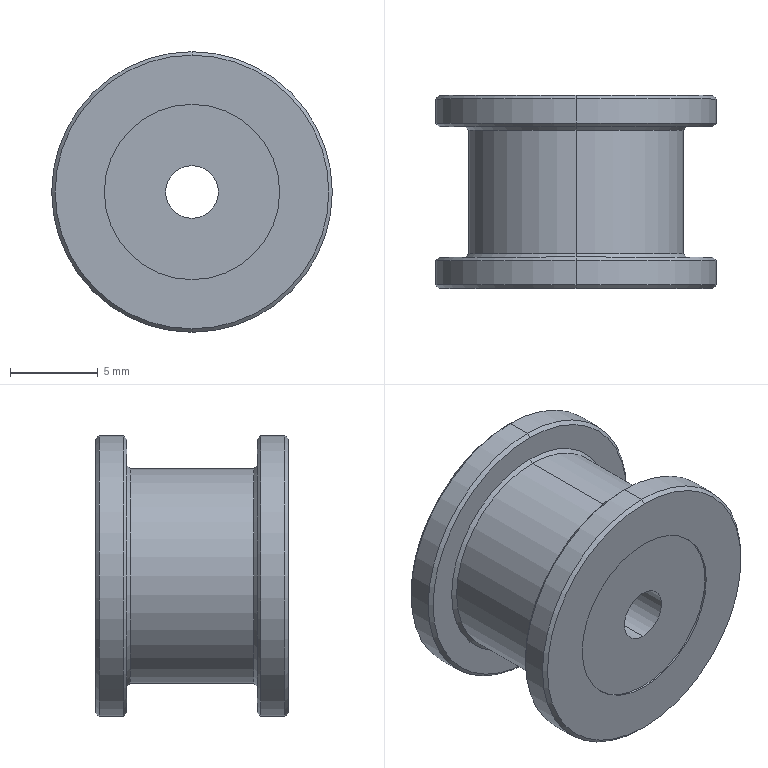Part | SolidWorks | features BaseBody 1 | 1 solid | 30 faces | box 16 x 11 x 16 mm | volume 1494 mm3 | cylinder 12 | cone 12 | plane 6 | commonest cylinder face diameters 10 x4 16 x4 3 x2 12.22 x2
STEP:
#1=CARTESIAN_POINT('',(-150.906,17.76,6.11));
#2=VERTEX_POINT('',#1);
#3=CARTESIAN_POINT('',(-150.906,17.76,-6.11));
#4=VERTEX_POINT('',#3);
#5=CARTESIAN_POINT('',(-150.906,17.76,0.));
#6=DIRECTION('',(0.,1.,0.));
#7=DIRECTION('',(0.,0.,1.));
#8=AXIS2_PLACEMENT_3D('',#5,#6,#7);
#9=CIRCLE('',#8,6.11);
#10=EDGE_CURVE('',#2,#4,#9,.T.);
#11=ORIENTED_EDGE('',*,*,#10,.T.);
#12=CARTESIAN_POINT('',(-150.906,24.8,-6.11));
#13=VERTEX_POINT('',#12);
#14=CARTESIAN_POINT('',(-150.906,21.28,-6.11));
#15=DIRECTION('',(0.,1.,0.));
#16=VECTOR('',#15,1000.);
#17=LINE('',#14,#16);
#18=EDGE_CURVE('',#4,#13,#17,.T.);
#19=ORIENTED_EDGE('',*,*,#18,.T.);
#20=CARTESIAN_POINT('',(-150.906,24.8,6.11));
#21=VERTEX_POINT('',#20);
#22=CARTESIAN_POINT('',(-150.906,24.8,0.));
#23=DIRECTION('',(0.,-1.,0.));
#24=DIRECTION('',(0.,0.,1.));
#25=AXIS2_PLACEMENT_3D('',#22,#23,#24);
#26=CIRCLE('',#25,6.11);
#27=EDGE_CURVE('',#13,#21,#26,.T.);
#28=ORIENTED_EDGE('',*,*,#27,.T.);
#29=CARTESIAN_POINT('',(-150.906,21.28,6.11));
#30=DIRECTION('',(0.,1.,0.));
#31=VECTOR('',#30,1000.);
#32=LINE('',#29,#31);
#33=EDGE_CURVE('',#2,#21,#32,.T.);
#34=ORIENTED_EDGE('',*,*,#33,.F.);
#35=EDGE_LOOP('',(#11,#19,#28,#34));
#36=FACE_OUTER_BOUND('',#35,.T.);
#37=CARTESIAN_POINT('',(-150.906,21.28,0.));
#38=DIRECTION('',(0.,1.,0.));
#39=DIRECTION('',(0.,0.,1.));
#40=AXIS2_PLACEMENT_3D('',#37,#38,#39);
#41=CYLINDRICAL_SURFACE('',#40,6.11);
#42=ADVANCED_FACE('',(#36),#41,.T.);
#43=ORIENTED_EDGE('',*,*,#10,.F.);
#44=CARTESIAN_POINT('',(-150.906,17.56,6.31));
#45=VERTEX_POINT('',#44);
#46=CARTESIAN_POINT('',(-150.906,17.56,6.31));
#47=DIRECTION('',(0.,-0.7071,0.7071));
#48=VECTOR('',#47,1000.);
#49=LINE('',#46,#48);
#50=EDGE_CURVE('',#2,#45,#49,.T.);
#51=ORIENTED_EDGE('',*,*,#50,.T.);
#52=CARTESIAN_POINT('',(-150.906,17.56,-6.31));
#53=VERTEX_POINT('',#52);
#54=CARTESIAN_POINT('',(-150.906,17.56,0.));
#55=DIRECTION('',(0.,1.,0.));
#56=DIRECTION('',(0.,0.,-1.));
#57=AXIS2_PLACEMENT_3D('',#54,#55,#56);
#58=CIRCLE('',#57,6.31);
#59=EDGE_CURVE('',#45,#53,#58,.T.);
#60=ORIENTED_EDGE('',*,*,#59,.T.);
#61=CARTESIAN_POINT('',(-150.906,17.56,-6.31));
#62=DIRECTION('',(0.,-0.7071,-0.7071));
#63=VECTOR('',#62,1000.);
#64=LINE('',#61,#63);
#65=EDGE_CURVE('',#4,#53,#64,.T.);
#66=ORIENTED_EDGE('',*,*,#65,.F.);
#67=EDGE_LOOP('',(#43,#51,#60,#66));
#68=FACE_OUTER_BOUND('',#67,.T.);
#69=CARTESIAN_POINT('',(-150.906,17.56,0.));
#70=DIRECTION('',(0.,-1.,0.));
#71=DIRECTION('',(0.,0.,-1.));
#72=AXIS2_PLACEMENT_3D('',#69,#70,#71);
#73=CONICAL_SURFACE('',#72,6.31,0.7854);
#74=ADVANCED_FACE('',(#68),#73,.T.);
#75=ORIENTED_EDGE('',*,*,#27,.F.);
#76=CARTESIAN_POINT('',(-150.906,25.,-6.31));
#77=VERTEX_POINT('',#76);
#78=CARTESIAN_POINT('',(-150.906,25.,-6.31));
#79=DIRECTION('',(0.,0.7071,-0.7071));
#80=VECTOR('',#79,1000.);
#81=LINE('',#78,#80);
#82=EDGE_CURVE('',#13,#77,#81,.T.);
#83=ORIENTED_EDGE('',*,*,#82,.T.);
#84=CARTESIAN_POINT('',(-150.906,25.,6.31));
#85=VERTEX_POINT('',#84);
#86=CARTESIAN_POINT('',(-150.906,25.,0.));
#87=DIRECTION('',(0.,-1.,0.));
#88=DIRECTION('',(0.,0.,1.));
#89=AXIS2_PLACEMENT_3D('',#86,#87,#88);
#90=CIRCLE('',#89,6.31);
#91=EDGE_CURVE('',#77,#85,#90,.T.);
#92=ORIENTED_EDGE('',*,*,#91,.T.);
#93=CARTESIAN_POINT('',(-150.906,25.,6.31));
#94=DIRECTION('',(0.,0.7071,0.7071));
#95=VECTOR('',#94,1000.);
#96=LINE('',#93,#95);
#97=EDGE_CURVE('',#21,#85,#96,.T.);
#98=ORIENTED_EDGE('',*,*,#97,.F.);
#99=EDGE_LOOP('',(#75,#83,#92,#98));
#100=FACE_OUTER_BOUND('',#99,.T.);
#101=CARTESIAN_POINT('',(-150.906,25.,0.));
#102=DIRECTION('',(0.,1.,0.));
#103=DIRECTION('',(0.,0.,1.));
#104=AXIS2_PLACEMENT_3D('',#101,#102,#103);
#105=CONICAL_SURFACE('',#104,6.31,0.7854);
#106=ADVANCED_FACE('',(#100),#105,.T.);
#107=CARTESIAN_POINT('',(-150.906,17.56,7.8));
#108=VERTEX_POINT('',#107);
#109=CARTESIAN_POINT('',(-150.906,17.56,-7.8));
#110=VERTEX_POINT('',#109);
#111=CARTESIAN_POINT('',(-150.906,17.56,0.));
#112=DIRECTION('',(0.,1.,0.));
#113=DIRECTION('',(0.,0.,-1.));
#114=AXIS2_PLACEMENT_3D('',#111,#112,#113);
#115=CIRCLE('',#114,7.8);
#116=EDGE_CURVE('',#108,#110,#115,.T.);
#117=ORIENTED_EDGE('',*,*,#116,.F.);
#118=CARTESIAN_POINT('',(-150.906,17.36,8.));
#119=VERTEX_POINT('',#118);
#120=CARTESIAN_POINT('',(-150.906,17.36,8.));
#121=DIRECTION('',(0.,-0.7071,0.7071));
#122=VECTOR('',#121,1000.);
#123=LINE('',#120,#122);
#124=EDGE_CURVE('',#108,#119,#123,.T.);
#125=ORIENTED_EDGE('',*,*,#124,.T.);
#126=CARTESIAN_POINT('',(-150.906,17.36,-8.));
#127=VERTEX_POINT('',#126);
#128=CARTESIAN_POINT('',(-150.906,17.36,0.));
#129=DIRECTION('',(0.,1.,0.));
#130=DIRECTION('',(-1.,0.,0.));
#131=AXIS2_PLACEMENT_3D('',#128,#129,#130);
#132=CIRCLE('',#131,8.);
#133=EDGE_CURVE('',#119,#127,#132,.T.);
#134=ORIENTED_EDGE('',*,*,#133,.T.);
#135=CARTESIAN_POINT('',(-150.906,17.36,-8.));
#136=DIRECTION('',(0.,-0.7071,-0.7071));
#137=VECTOR('',#136,1000.);
#138=LINE('',#135,#137);
#139=EDGE_CURVE('',#110,#127,#138,.T.);
#140=ORIENTED_EDGE('',*,*,#139,.F.);
#141=EDGE_LOOP('',(#117,#125,#134,#140));
#142=FACE_OUTER_BOUND('',#141,.T.);
#143=CARTESIAN_POINT('',(-150.906,17.36,0.));
#144=DIRECTION('',(0.,-1.,0.));
#145=DIRECTION('',(0.,0.,-1.));
#146=AXIS2_PLACEMENT_3D('',#143,#144,#145);
#147=CONICAL_SURFACE('',#146,8.,0.7854);
#148=ADVANCED_FACE('',(#142),#147,.T.);
#149=CARTESIAN_POINT('',(-150.906,25.,-7.8));
#150=VERTEX_POINT('',#149);
#151=CARTESIAN_POINT('',(-150.906,25.,7.8));
#152=VERTEX_POINT('',#151);
#153=CARTESIAN_POINT('',(-150.906,25.,0.));
#154=DIRECTION('',(0.,-1.,0.));
#155=DIRECTION('',(0.,0.,1.));
#156=AXIS2_PLACEMENT_3D('',#153,#154,#155);
#157=CIRCLE('',#156,7.8);
#158=EDGE_CURVE('',#150,#152,#157,.T.);
#159=ORIENTED_EDGE('',*,*,#158,.F.);
#160=CARTESIAN_POINT('',(-150.906,25.2,-8.));
#161=VERTEX_POINT('',#160);
#162=CARTESIAN_POINT('',(-150.906,25.2,-8.));
#163=DIRECTION('',(0.,0.7071,-0.7071));
#164=VECTOR('',#163,1000.);
#165=LINE('',#162,#164);
#166=EDGE_CURVE('',#150,#161,#165,.T.);
#167=ORIENTED_EDGE('',*,*,#166,.T.);
#168=CARTESIAN_POINT('',(-150.906,25.2,8.));
#169=VERTEX_POINT('',#168);
#170=CARTESIAN_POINT('',(-150.906,25.2,0.));
#171=DIRECTION('',(0.,-1.,0.));
#172=DIRECTION('',(-1.,0.,0.));
#173=AXIS2_PLACEMENT_3D('',#170,#171,#172);
#174=CIRCLE('',#173,8.);
#175=EDGE_CURVE('',#161,#169,#174,.T.);
#176=ORIENTED_EDGE('',*,*,#175,.T.);
#177=CARTESIAN_POINT('',(-150.906,25.2,8.));
#178=DIRECTION('',(0.,0.7071,0.7071));
#179=VECTOR('',#178,1000.);
#180=LINE('',#177,#179);
#181=EDGE_CURVE('',#152,#169,#180,.T.);
#182=ORIENTED_EDGE('',*,*,#181,.F.);
#183=EDGE_LOOP('',(#159,#167,#176,#182));
#184=FACE_OUTER_BOUND('',#183,.T.);
#185=CARTESIAN_POINT('',(-150.906,25.2,0.));
#186=DIRECTION('',(0.,1.,0.));
#187=DIRECTION('',(0.,0.,1.));
#188=AXIS2_PLACEMENT_3D('',#185,#186,#187);
#189=CONICAL_SURFACE('',#188,8.,0.7854);
#190=ADVANCED_FACE('',(#184),#189,.T.);
#191=CARTESIAN_POINT('',(-150.906,15.98,8.));
#192=VERTEX_POINT('',#191);
#193=CARTESIAN_POINT('',(-150.906,15.98,-8.));
#194=VERTEX_POINT('',#193);
#195=CARTESIAN_POINT('',(-150.906,15.98,0.));
#196=DIRECTION('',(0.,1.,0.));
#197=DIRECTION('',(0.,0.,1.));
#198=AXIS2_PLACEMENT_3D('',#195,#196,#197);
#199=CIRCLE('',#198,8.);
#200=EDGE_CURVE('',#192,#194,#199,.T.);
#201=ORIENTED_EDGE('',*,*,#200,.T.);
#202=CARTESIAN_POINT('',(-150.906,16.67,-8.));
#203=DIRECTION('',(0.,1.,0.));
#204=VECTOR('',#203,1000.);
#205=LINE('',#202,#204);
#206=EDGE_CURVE('',#194,#127,#205,.T.);
#207=ORIENTED_EDGE('',*,*,#206,.T.);
#208=ORIENTED_EDGE('',*,*,#133,.F.);
#209=CARTESIAN_POINT('',(-150.906,16.67,8.));
#210=DIRECTION('',(0.,1.,0.));
#211=VECTOR('',#210,1000.);
#212=LINE('',#209,#211);
#213=EDGE_CURVE('',#192,#119,#212,.T.);
#214=ORIENTED_EDGE('',*,*,#213,.F.);
#215=EDGE_LOOP('',(#201,#207,#208,#214));
#216=FACE_OUTER_BOUND('',#215,.T.);
#217=CARTESIAN_POINT('',(-150.906,16.67,0.));
#218=DIRECTION('',(0.,1.,0.));
#219=DIRECTION('',(0.,0.,1.));
#220=AXIS2_PLACEMENT_3D('',#217,#218,#219);
#221=CYLINDRICAL_SURFACE('',#220,8.);
#222=ADVANCED_FACE('',(#216),#221,.T.);
#223=ORIENTED_EDGE('',*,*,#175,.F.);
#224=CARTESIAN_POINT('',(-150.906,26.58,-8.));
#225=VERTEX_POINT('',#224);
#226=CARTESIAN_POINT('',(-150.906,25.89,-8.));
#227=DIRECTION('',(0.,1.,0.));
#228=VECTOR('',#227,1000.);
#229=LINE('',#226,#228);
#230=EDGE_CURVE('',#161,#225,#229,.T.);
#231=ORIENTED_EDGE('',*,*,#230,.T.);
#232=CARTESIAN_POINT('',(-150.906,26.58,8.));
#233=VERTEX_POINT('',#232);
#234=CARTESIAN_POINT('',(-150.906,26.58,0.));
#235=DIRECTION('',(0.,-1.,0.));
#236=DIRECTION('',(0.,0.,1.));
#237=AXIS2_PLACEMENT_3D('',#234,#235,#236);
#238=CIRCLE('',#237,8.);
#239=EDGE_CURVE('',#225,#233,#238,.T.);
#240=ORIENTED_EDGE('',*,*,#239,.T.);
#241=CARTESIAN_POINT('',(-150.906,25.89,8.));
#242=DIRECTION('',(0.,1.,0.));
#243=VECTOR('',#242,1000.);
#244=LINE('',#241,#243);
#245=EDGE_CURVE('',#169,#233,#244,.T.);
#246=ORIENTED_EDGE('',*,*,#245,.F.);
#247=EDGE_LOOP('',(#223,#231,#240,#246));
#248=FACE_OUTER_BOUND('',#247,.T.);
#249=CARTESIAN_POINT('',(-150.906,25.89,0.));
#250=DIRECTION('',(0.,1.,0.));
#251=DIRECTION('',(0.,0.,1.));
#252=AXIS2_PLACEMENT_3D('',#249,#250,#251);
#253=CYLINDRICAL_SURFACE('',#252,8.);
#254=ADVANCED_FACE('',(#248),#253,.T.);
#255=CARTESIAN_POINT('',(-150.906,15.78,7.8));
#256=VERTEX_POINT('',#255);
#257=CARTESIAN_POINT('',(-150.906,15.78,-7.8));
#258=VERTEX_POINT('',#257);
#259=CARTESIAN_POINT('',(-150.906,15.78,0.));
#260=DIRECTION('',(0.,1.,0.));
#261=DIRECTION('',(0.,0.,1.));
#262=AXIS2_PLACEMENT_3D('',#259,#260,#261);
#263=CIRCLE('',#262,7.8);
#264=EDGE_CURVE('',#256,#258,#263,.T.);
#265=ORIENTED_EDGE('',*,*,#264,.T.);
#266=CARTESIAN_POINT('',(-150.906,15.98,-8.));
#267=DIRECTION('',(0.,0.7071,-0.7071));
#268=VECTOR('',#267,1000.);
#269=LINE('',#266,#268);
#270=EDGE_CURVE('',#258,#194,#269,.T.);
#271=ORIENTED_EDGE('',*,*,#270,.T.);
#272=ORIENTED_EDGE('',*,*,#200,.F.);
#273=CARTESIAN_POINT('',(-150.906,15.98,8.));
#274=DIRECTION('',(0.,0.7071,0.7071));
#275=VECTOR('',#274,1000.);
#276=LINE('',#273,#275);
#277=EDGE_CURVE('',#256,#192,#276,.T.);
#278=ORIENTED_EDGE('',*,*,#277,.F.);
#279=EDGE_LOOP('',(#265,#271,#272,#278));
#280=FACE_OUTER_BOUND('',#279,.T.);
#281=CARTESIAN_POINT('',(-150.906,15.98,0.));
#282=DIRECTION('',(0.,1.,0.));
#283=DIRECTION('',(0.,0.,1.));
#284=AXIS2_PLACEMENT_3D('',#281,#282,#283);
#285=CONICAL_SURFACE('',#284,8.,0.7854);
#286=ADVANCED_FACE('',(#280),#285,.T.);
#287=CARTESIAN_POINT('',(-150.906,26.78,-7.8));
#288=VERTEX_POINT('',#287);
#289=CARTESIAN_POINT('',(-150.906,26.78,7.8));
#290=VERTEX_POINT('',#289);
#291=CARTESIAN_POINT('',(-150.906,26.78,0.));
#292=DIRECTION('',(0.,-1.,0.));
#293=DIRECTION('',(0.,0.,-1.));
#294=AXIS2_PLACEMENT_3D('',#291,#292,#293);
#295=CIRCLE('',#294,7.8);
#296=EDGE_CURVE('',#288,#290,#295,.T.);
#297=ORIENTED_EDGE('',*,*,#296,.T.);
#298=CARTESIAN_POINT('',(-150.906,26.58,8.));
#299=DIRECTION('',(0.,-0.7071,0.7071));
#300=VECTOR('',#299,1000.);
#301=LINE('',#298,#300);
#302=EDGE_CURVE('',#290,#233,#301,.T.);
#303=ORIENTED_EDGE('',*,*,#302,.T.);
#304=ORIENTED_EDGE('',*,*,#239,.F.);
#305=CARTESIAN_POINT('',(-150.906,26.58,-8.));
#306=DIRECTION('',(0.,-0.7071,-0.7071));
#307=VECTOR('',#306,1000.);
#308=LINE('',#305,#307);
#309=EDGE_CURVE('',#288,#225,#308,.T.);
#310=ORIENTED_EDGE('',*,*,#309,.F.);
#311=EDGE_LOOP('',(#297,#303,#304,#310));
#312=FACE_OUTER_BOUND('',#311,.T.);
#313=CARTESIAN_POINT('',(-150.906,26.58,0.));
#314=DIRECTION('',(0.,-1.,0.));
#315=DIRECTION('',(0.,0.,-1.));
#316=AXIS2_PLACEMENT_3D('',#313,#314,#315);
#317=CONICAL_SURFACE('',#316,8.,0.7854);
#318=ADVANCED_FACE('',(#312),#317,.T.);
#319=CARTESIAN_POINT('',(-150.906,15.78,-5.));
#320=VERTEX_POINT('',#319);
#321=CARTESIAN_POINT('',(-150.906,15.78,5.));
#322=VERTEX_POINT('',#321);
#323=CARTESIAN_POINT('',(-150.906,15.78,0.));
#324=DIRECTION('',(0.,1.,0.));
#325=DIRECTION('',(0.,0.,1.));
#326=AXIS2_PLACEMENT_3D('',#323,#324,#325);
#327=CIRCLE('',#326,5.);
#328=EDGE_CURVE('',#320,#322,#327,.T.);
#329=ORIENTED_EDGE('',*,*,#328,.F.);
#330=CARTESIAN_POINT('',(-150.906,15.88,-5.));
#331=VERTEX_POINT('',#330);
#332=CARTESIAN_POINT('',(-150.906,15.78,-5.));
#333=DIRECTION('',(0.,1.,0.));
#334=VECTOR('',#333,1000.);
#335=LINE('',#332,#334);
#336=EDGE_CURVE('',#320,#331,#335,.T.);
#337=ORIENTED_EDGE('',*,*,#336,.T.);
#338=CARTESIAN_POINT('',(-150.906,15.88,5.));
#339=VERTEX_POINT('',#338);
#340=CARTESIAN_POINT('',(-150.906,15.88,0.));
#341=DIRECTION('',(0.,-1.,0.));
#342=DIRECTION('',(0.,0.,1.));
#343=AXIS2_PLACEMENT_3D('',#340,#341,#342);
#344=CIRCLE('',#343,5.);
#345=EDGE_CURVE('',#339,#331,#344,.T.);
#346=ORIENTED_EDGE('',*,*,#345,.F.);
#347=CARTESIAN_POINT('',(-150.906,15.78,5.));
#348=DIRECTION('',(0.,1.,0.));
#349=VECTOR('',#348,1000.);
#350=LINE('',#347,#349);
#351=EDGE_CURVE('',#322,#339,#350,.T.);
#352=ORIENTED_EDGE('',*,*,#351,.F.);
#353=EDGE_LOOP('',(#329,#337,#346,#352));
#354=FACE_OUTER_BOUND('',#353,.T.);
#355=CARTESIAN_POINT('',(-150.906,15.78,0.));
#356=DIRECTION('',(0.,1.,0.));
#357=DIRECTION('',(0.,0.,1.));
#358=AXIS2_PLACEMENT_3D('',#355,#356,#357);
#359=CYLINDRICAL_SURFACE('',#358,5.);
#360=ADVANCED_FACE('',(#354),#359,.F.);
#361=CARTESIAN_POINT('',(-150.906,26.78,5.));
#362=VERTEX_POINT('',#361);
#363=CARTESIAN_POINT('',(-150.906,26.78,-5.));
#364=VERTEX_POINT('',#363);
#365=CARTESIAN_POINT('',(-150.906,26.78,0.));
#366=DIRECTION('',(0.,-1.,0.));
#367=DIRECTION('',(0.,0.,-1.));
#368=AXIS2_PLACEMENT_3D('',#365,#366,#367);
#369=CIRCLE('',#368,5.);
#370=EDGE_CURVE('',#362,#364,#369,.T.);
#371=ORIENTED_EDGE('',*,*,#370,.F.);
#372=CARTESIAN_POINT('',(-150.906,26.68,5.));
#373=VERTEX_POINT('',#372);
#374=CARTESIAN_POINT('',(-150.906,26.78,5.));
#375=DIRECTION('',(0.,-1.,0.));
#376=VECTOR('',#375,1000.);
#377=LINE('',#374,#376);
#378=EDGE_CURVE('',#362,#373,#377,.T.);
#379=ORIENTED_EDGE('',*,*,#378,.T.);
#380=CARTESIAN_POINT('',(-150.906,26.68,-5.));
#381=VERTEX_POINT('',#380);
#382=CARTESIAN_POINT('',(-150.906,26.68,0.));
#383=DIRECTION('',(0.,1.,0.));
#384=DIRECTION('',(0.,0.,-1.));
#385=AXIS2_PLACEMENT_3D('',#382,#383,#384);
#386=CIRCLE('',#385,5.);
#387=EDGE_CURVE('',#381,#373,#386,.T.);
#388=ORIENTED_EDGE('',*,*,#387,.F.);
#389=CARTESIAN_POINT('',(-150.906,26.78,-5.));
#390=DIRECTION('',(0.,-1.,0.));
#391=VECTOR('',#390,1000.);
#392=LINE('',#389,#391);
#393=EDGE_CURVE('',#364,#381,#392,.T.);
#394=ORIENTED_EDGE('',*,*,#393,.F.);
#395=EDGE_LOOP('',(#371,#379,#388,#394));
#396=FACE_OUTER_BOUND('',#395,.T.);
#397=CARTESIAN_POINT('',(-150.906,26.78,0.));
#398=DIRECTION('',(0.,-1.,0.));
#399=DIRECTION('',(0.,0.,-1.));
#400=AXIS2_PLACEMENT_3D('',#397,#398,#399);
#401=CYLINDRICAL_SURFACE('',#400,5.);
#402=ADVANCED_FACE('',(#396),#401,.F.);
#403=CARTESIAN_POINT('',(-150.906,15.88,1.5));
#404=VERTEX_POINT('',#403);
#405=CARTESIAN_POINT('',(-150.906,15.88,-1.5));
#406=VERTEX_POINT('',#405);
#407=CARTESIAN_POINT('',(-150.906,15.88,0.));
#408=DIRECTION('',(0.,-1.,0.));
#409=DIRECTION('',(0.,0.,1.));
#410=AXIS2_PLACEMENT_3D('',#407,#408,#409);
#411=CIRCLE('',#410,1.5);
#412=EDGE_CURVE('',#404,#406,#411,.T.);
#413=ORIENTED_EDGE('',*,*,#412,.T.);
#414=CARTESIAN_POINT('',(-150.906,26.68,-1.5));
#415=VERTEX_POINT('',#414);
#416=CARTESIAN_POINT('',(-150.906,21.28,-1.5));
#417=DIRECTION('',(0.,1.,0.));
#418=VECTOR('',#417,1000.);
#419=LINE('',#416,#418);
#420=EDGE_CURVE('',#406,#415,#419,.T.);
#421=ORIENTED_EDGE('',*,*,#420,.T.);
#422=CARTESIAN_POINT('',(-150.906,26.68,1.5));
#423=VERTEX_POINT('',#422);
#424=CARTESIAN_POINT('',(-150.906,26.68,0.));
#425=DIRECTION('',(0.,1.,0.));
#426=DIRECTION('',(0.,0.,1.));
#427=AXIS2_PLACEMENT_3D('',#424,#425,#426);
#428=CIRCLE('',#427,1.5);
#429=EDGE_CURVE('',#415,#423,#428,.T.);
#430=ORIENTED_EDGE('',*,*,#429,.T.);
#431=CARTESIAN_POINT('',(-150.906,21.28,1.5));
#432=DIRECTION('',(0.,1.,0.));
#433=VECTOR('',#432,1000.);
#434=LINE('',#431,#433);
#435=EDGE_CURVE('',#404,#423,#434,.T.);
#436=ORIENTED_EDGE('',*,*,#435,.F.);
#437=EDGE_LOOP('',(#413,#421,#430,#436));
#438=FACE_OUTER_BOUND('',#437,.T.);
#439=CARTESIAN_POINT('',(-150.906,21.28,0.));
#440=DIRECTION('',(0.,1.,0.));
#441=DIRECTION('',(0.,0.,1.));
#442=AXIS2_PLACEMENT_3D('',#439,#440,#441);
#443=CYLINDRICAL_SURFACE('',#442,1.5);
#444=ADVANCED_FACE('',(#438),#443,.F.);
#445=ORIENTED_EDGE('',*,*,#18,.F.);
#446=CARTESIAN_POINT('',(-150.906,17.76,0.));
#447=DIRECTION('',(0.,1.,0.));
#448=DIRECTION('',(0.,0.,1.));
#449=AXIS2_PLACEMENT_3D('',#446,#447,#448);
#450=CIRCLE('',#449,6.11);
#451=EDGE_CURVE('',#4,#2,#450,.T.);
#452=ORIENTED_EDGE('',*,*,#451,.T.);
#453=ORIENTED_EDGE('',*,*,#33,.T.);
#454=CARTESIAN_POINT('',(-150.906,24.8,0.));
#455=DIRECTION('',(0.,-1.,0.));
#456=DIRECTION('',(0.,0.,1.));
#457=AXIS2_PLACEMENT_3D('',#454,#455,#456);
#458=CIRCLE('',#457,6.11);
#459=EDGE_CURVE('',#21,#13,#458,.T.);
#460=ORIENTED_EDGE('',*,*,#459,.T.);
#461=EDGE_LOOP('',(#445,#452,#453,#460));
#462=FACE_OUTER_BOUND('',#461,.T.);
#463=CARTESIAN_POINT('',(-150.906,21.28,0.));
#464=DIRECTION('',(0.,1.,0.));
#465=DIRECTION('',(0.,0.,1.));
#466=AXIS2_PLACEMENT_3D('',#463,#464,#465);
#467=CYLINDRICAL_SURFACE('',#466,6.11);
#468=ADVANCED_FACE('',(#462),#467,.T.);
#469=ORIENTED_EDGE('',*,*,#50,.F.);
#470=ORIENTED_EDGE('',*,*,#451,.F.);
#471=ORIENTED_EDGE('',*,*,#65,.T.);
#472=CARTESIAN_POINT('',(-150.906,17.56,0.));
#473=DIRECTION('',(0.,1.,0.));
#474=DIRECTION('',(0.,0.,-1.));
#475=AXIS2_PLACEMENT_3D('',#472,#473,#474);
#476=CIRCLE('',#475,6.31);
#477=EDGE_CURVE('',#53,#45,#476,.T.);
#478=ORIENTED_EDGE('',*,*,#477,.T.);
#479=EDGE_LOOP('',(#469,#470,#471,#478));
#480=FACE_OUTER_BOUND('',#479,.T.);
#481=CARTESIAN_POINT('',(-150.906,17.56,0.));
#482=DIRECTION('',(0.,-1.,0.));
#483=DIRECTION('',(0.,0.,-1.));
#484=AXIS2_PLACEMENT_3D('',#481,#482,#483);
#485=CONICAL_SURFACE('',#484,6.31,0.7854);
#486=ADVANCED_FACE('',(#480),#485,.T.);
#487=ORIENTED_EDGE('',*,*,#82,.F.);
#488=ORIENTED_EDGE('',*,*,#459,.F.);
#489=ORIENTED_EDGE('',*,*,#97,.T.);
#490=CARTESIAN_POINT('',(-150.906,25.,0.));
#491=DIRECTION('',(0.,-1.,0.));
#492=DIRECTION('',(0.,0.,1.));
#493=AXIS2_PLACEMENT_3D('',#490,#491,#492);
#494=CIRCLE('',#493,6.31);
#495=EDGE_CURVE('',#85,#77,#494,.T.);
#496=ORIENTED_EDGE('',*,*,#495,.T.);
#497=EDGE_LOOP('',(#487,#488,#489,#496));
#498=FACE_OUTER_BOUND('',#497,.T.);
#499=CARTESIAN_POINT('',(-150.906,25.,0.));
#500=DIRECTION('',(0.,1.,0.));
#501=DIRECTION('',(0.,0.,1.));
#502=AXIS2_PLACEMENT_3D('',#499,#500,#501);
#503=CONICAL_SURFACE('',#502,6.31,0.7854);
#504=ADVANCED_FACE('',(#498),#503,.T.);
#505=ORIENTED_EDGE('',*,*,#477,.F.);
#506=ORIENTED_EDGE('',*,*,#59,.F.);
#507=EDGE_LOOP('',(#505,#506));
#508=FACE_BOUND('',#507,.T.);
#509=CARTESIAN_POINT('',(-150.906,17.56,0.));
#510=DIRECTION('',(0.,1.,0.));
#511=DIRECTION('',(0.,0.,-1.));
#512=AXIS2_PLACEMENT_3D('',#509,#510,#511);
#513=CIRCLE('',#512,7.8);
#514=EDGE_CURVE('',#110,#108,#513,.T.);
#515=ORIENTED_EDGE('',*,*,#514,.T.);
#516=ORIENTED_EDGE('',*,*,#116,.T.);
#517=EDGE_LOOP('',(#515,#516));
#518=FACE_OUTER_BOUND('',#517,.T.);
#519=CARTESIAN_POINT('',(-157.961,17.56,0.));
#520=DIRECTION('',(0.,1.,0.));
#521=DIRECTION('',(0.,0.,1.));
#522=AXIS2_PLACEMENT_3D('',#519,#520,#521);
#523=PLANE('',#522);
#524=ADVANCED_FACE('',(#508,#518),#523,.T.);
#525=ORIENTED_EDGE('',*,*,#495,.F.);
#526=ORIENTED_EDGE('',*,*,#91,.F.);
#527=EDGE_LOOP('',(#525,#526));
#528=FACE_BOUND('',#527,.T.);
#529=CARTESIAN_POINT('',(-150.906,25.,0.));
#530=DIRECTION('',(0.,-1.,0.));
#531=DIRECTION('',(0.,0.,1.));
#532=AXIS2_PLACEMENT_3D('',#529,#530,#531);
#533=CIRCLE('',#532,7.8);
#534=EDGE_CURVE('',#152,#150,#533,.T.);
#535=ORIENTED_EDGE('',*,*,#534,.T.);
#536=ORIENTED_EDGE('',*,*,#158,.T.);
#537=EDGE_LOOP('',(#535,#536));
#538=FACE_OUTER_BOUND('',#537,.T.);
#539=CARTESIAN_POINT('',(-157.961,25.,0.));
#540=DIRECTION('',(0.,-1.,0.));
#541=DIRECTION('',(0.,0.,-1.));
#542=AXIS2_PLACEMENT_3D('',#539,#540,#541);
#543=PLANE('',#542);
#544=ADVANCED_FACE('',(#528,#538),#543,.T.);
#545=ORIENTED_EDGE('',*,*,#124,.F.);
#546=ORIENTED_EDGE('',*,*,#514,.F.);
#547=ORIENTED_EDGE('',*,*,#139,.T.);
#548=CARTESIAN_POINT('',(-150.906,17.36,0.));
#549=DIRECTION('',(0.,1.,0.));
#550=DIRECTION('',(-1.,0.,0.));
#551=AXIS2_PLACEMENT_3D('',#548,#549,#550);
#552=CIRCLE('',#551,8.);
#553=EDGE_CURVE('',#127,#119,#552,.T.);
#554=ORIENTED_EDGE('',*,*,#553,.T.);
#555=EDGE_LOOP('',(#545,#546,#547,#554));
#556=FACE_OUTER_BOUND('',#555,.T.);
#557=CARTESIAN_POINT('',(-150.906,17.36,0.));
#558=DIRECTION('',(0.,-1.,0.));
#559=DIRECTION('',(0.,0.,-1.));
#560=AXIS2_PLACEMENT_3D('',#557,#558,#559);
#561=CONICAL_SURFACE('',#560,8.,0.7854);
#562=ADVANCED_FACE('',(#556),#561,.T.);
#563=ORIENTED_EDGE('',*,*,#166,.F.);
#564=ORIENTED_EDGE('',*,*,#534,.F.);
#565=ORIENTED_EDGE('',*,*,#181,.T.);
#566=CARTESIAN_POINT('',(-150.906,25.2,0.));
#567=DIRECTION('',(0.,-1.,0.));
#568=DIRECTION('',(-1.,0.,0.));
#569=AXIS2_PLACEMENT_3D('',#566,#567,#568);
#570=CIRCLE('',#569,8.);
#571=EDGE_CURVE('',#169,#161,#570,.T.);
#572=ORIENTED_EDGE('',*,*,#571,.T.);
#573=EDGE_LOOP('',(#563,#564,#565,#572));
#574=FACE_OUTER_BOUND('',#573,.T.);
#575=CARTESIAN_POINT('',(-150.906,25.2,0.));
#576=DIRECTION('',(0.,1.,0.));
#577=DIRECTION('',(0.,0.,1.));
#578=AXIS2_PLACEMENT_3D('',#575,#576,#577);
#579=CONICAL_SURFACE('',#578,8.,0.7854);
#580=ADVANCED_FACE('',(#574),#579,.T.);
#581=ORIENTED_EDGE('',*,*,#206,.F.);
#582=CARTESIAN_POINT('',(-150.906,15.98,0.));
#583=DIRECTION('',(0.,1.,0.));
#584=DIRECTION('',(0.,0.,1.));
#585=AXIS2_PLACEMENT_3D('',#582,#583,#584);
#586=CIRCLE('',#585,8.);
#587=EDGE_CURVE('',#194,#192,#586,.T.);
#588=ORIENTED_EDGE('',*,*,#587,.T.);
#589=ORIENTED_EDGE('',*,*,#213,.T.);
#590=ORIENTED_EDGE('',*,*,#553,.F.);
#591=EDGE_LOOP('',(#581,#588,#589,#590));
#592=FACE_OUTER_BOUND('',#591,.T.);
#593=CARTESIAN_POINT('',(-150.906,16.67,0.));
#594=DIRECTION('',(0.,1.,0.));
#595=DIRECTION('',(0.,0.,1.));
#596=AXIS2_PLACEMENT_3D('',#593,#594,#595);
#597=CYLINDRICAL_SURFACE('',#596,8.);
#598=ADVANCED_FACE('',(#592),#597,.T.);
#599=ORIENTED_EDGE('',*,*,#230,.F.);
#600=ORIENTED_EDGE('',*,*,#571,.F.);
#601=ORIENTED_EDGE('',*,*,#245,.T.);
#602=CARTESIAN_POINT('',(-150.906,26.58,0.));
#603=DIRECTION('',(0.,-1.,0.));
#604=DIRECTION('',(0.,0.,1.));
#605=AXIS2_PLACEMENT_3D('',#602,#603,#604);
#606=CIRCLE('',#605,8.);
#607=EDGE_CURVE('',#233,#225,#606,.T.);
#608=ORIENTED_EDGE('',*,*,#607,.T.);
#609=EDGE_LOOP('',(#599,#600,#601,#608));
#610=FACE_OUTER_BOUND('',#609,.T.);
#611=CARTESIAN_POINT('',(-150.906,25.89,0.));
#612=DIRECTION('',(0.,1.,0.));
#613=DIRECTION('',(0.,0.,1.));
#614=AXIS2_PLACEMENT_3D('',#611,#612,#613);
#615=CYLINDRICAL_SURFACE('',#614,8.);
#616=ADVANCED_FACE('',(#610),#615,.T.);
#617=ORIENTED_EDGE('',*,*,#270,.F.);
#618=CARTESIAN_POINT('',(-150.906,15.78,0.));
#619=DIRECTION('',(0.,1.,0.));
#620=DIRECTION('',(0.,0.,1.));
#621=AXIS2_PLACEMENT_3D('',#618,#619,#620);
#622=CIRCLE('',#621,7.8);
#623=EDGE_CURVE('',#258,#256,#622,.T.);
#624=ORIENTED_EDGE('',*,*,#623,.T.);
#625=ORIENTED_EDGE('',*,*,#277,.T.);
#626=ORIENTED_EDGE('',*,*,#587,.F.);
#627=EDGE_LOOP('',(#617,#624,#625,#626));
#628=FACE_OUTER_BOUND('',#627,.T.);
#629=CARTESIAN_POINT('',(-150.906,15.98,0.));
#630=DIRECTION('',(0.,1.,0.));
#631=DIRECTION('',(0.,0.,1.));
#632=AXIS2_PLACEMENT_3D('',#629,#630,#631);
#633=CONICAL_SURFACE('',#632,8.,0.7854);
#634=ADVANCED_FACE('',(#628),#633,.T.);
#635=ORIENTED_EDGE('',*,*,#302,.F.);
#636=CARTESIAN_POINT('',(-150.906,26.78,0.));
#637=DIRECTION('',(0.,-1.,0.));
#638=DIRECTION('',(0.,0.,-1.));
#639=AXIS2_PLACEMENT_3D('',#636,#637,#638);
#640=CIRCLE('',#639,7.8);
#641=EDGE_CURVE('',#290,#288,#640,.T.);
#642=ORIENTED_EDGE('',*,*,#641,.T.);
#643=ORIENTED_EDGE('',*,*,#309,.T.);
#644=ORIENTED_EDGE('',*,*,#607,.F.);
#645=EDGE_LOOP('',(#635,#642,#643,#644));
#646=FACE_OUTER_BOUND('',#645,.T.);
#647=CARTESIAN_POINT('',(-150.906,26.58,0.));
#648=DIRECTION('',(0.,-1.,0.));
#649=DIRECTION('',(0.,0.,-1.));
#650=AXIS2_PLACEMENT_3D('',#647,#648,#649);
#651=CONICAL_SURFACE('',#650,8.,0.7854);
#652=ADVANCED_FACE('',(#646),#651,.T.);
#653=CARTESIAN_POINT('',(-150.906,15.78,0.));
#654=DIRECTION('',(0.,1.,0.));
#655=DIRECTION('',(0.,0.,1.));
#656=AXIS2_PLACEMENT_3D('',#653,#654,#655);
#657=CIRCLE('',#656,5.);
#658=EDGE_CURVE('',#322,#320,#657,.T.);
#659=ORIENTED_EDGE('',*,*,#658,.T.);
#660=ORIENTED_EDGE('',*,*,#328,.T.);
#661=EDGE_LOOP('',(#659,#660));
#662=FACE_BOUND('',#661,.T.);
#663=ORIENTED_EDGE('',*,*,#264,.F.);
#664=ORIENTED_EDGE('',*,*,#623,.F.);
#665=EDGE_LOOP('',(#663,#664));
#666=FACE_OUTER_BOUND('',#665,.T.);
#667=CARTESIAN_POINT('',(-155.556,15.78,0.));
#668=DIRECTION('',(0.,-1.,0.));
#669=DIRECTION('',(0.,0.,-1.));
#670=AXIS2_PLACEMENT_3D('',#667,#668,#669);
#671=PLANE('',#670);
#672=ADVANCED_FACE('',(#662,#666),#671,.T.);
#673=CARTESIAN_POINT('',(-150.906,26.78,0.));
#674=DIRECTION('',(0.,-1.,0.));
#675=DIRECTION('',(0.,0.,-1.));
#676=AXIS2_PLACEMENT_3D('',#673,#674,#675);
#677=CIRCLE('',#676,5.);
#678=EDGE_CURVE('',#364,#362,#677,.T.);
#679=ORIENTED_EDGE('',*,*,#678,.T.);
#680=ORIENTED_EDGE('',*,*,#370,.T.);
#681=EDGE_LOOP('',(#679,#680));
#682=FACE_BOUND('',#681,.T.);
#683=ORIENTED_EDGE('',*,*,#296,.F.);
#684=ORIENTED_EDGE('',*,*,#641,.F.);
#685=EDGE_LOOP('',(#683,#684));
#686=FACE_OUTER_BOUND('',#685,.T.);
#687=CARTESIAN_POINT('',(-155.556,26.78,0.));
#688=DIRECTION('',(0.,1.,0.));
#689=DIRECTION('',(0.,0.,1.));
#690=AXIS2_PLACEMENT_3D('',#687,#688,#689);
#691=PLANE('',#690);
#692=ADVANCED_FACE('',(#682,#686),#691,.T.);
#693=ORIENTED_EDGE('',*,*,#336,.F.);
#694=ORIENTED_EDGE('',*,*,#658,.F.);
#695=ORIENTED_EDGE('',*,*,#351,.T.);
#696=CARTESIAN_POINT('',(-150.906,15.88,0.));
#697=DIRECTION('',(0.,-1.,0.));
#698=DIRECTION('',(0.,0.,1.));
#699=AXIS2_PLACEMENT_3D('',#696,#697,#698);
#700=CIRCLE('',#699,5.);
#701=EDGE_CURVE('',#331,#339,#700,.T.);
#702=ORIENTED_EDGE('',*,*,#701,.F.);
#703=EDGE_LOOP('',(#693,#694,#695,#702));
#704=FACE_OUTER_BOUND('',#703,.T.);
#705=CARTESIAN_POINT('',(-150.906,15.78,0.));
#706=DIRECTION('',(0.,1.,0.));
#707=DIRECTION('',(0.,0.,1.));
#708=AXIS2_PLACEMENT_3D('',#705,#706,#707);
#709=CYLINDRICAL_SURFACE('',#708,5.);
#710=ADVANCED_FACE('',(#704),#709,.F.);
#711=ORIENTED_EDGE('',*,*,#378,.F.);
#712=ORIENTED_EDGE('',*,*,#678,.F.);
#713=ORIENTED_EDGE('',*,*,#393,.T.);
#714=CARTESIAN_POINT('',(-150.906,26.68,0.));
#715=DIRECTION('',(0.,1.,0.));
#716=DIRECTION('',(0.,0.,-1.));
#717=AXIS2_PLACEMENT_3D('',#714,#715,#716);
#718=CIRCLE('',#717,5.);
#719=EDGE_CURVE('',#373,#381,#718,.T.);
#720=ORIENTED_EDGE('',*,*,#719,.F.);
#721=EDGE_LOOP('',(#711,#712,#713,#720));
#722=FACE_OUTER_BOUND('',#721,.T.);
#723=CARTESIAN_POINT('',(-150.906,26.78,0.));
#724=DIRECTION('',(0.,-1.,0.));
#725=DIRECTION('',(0.,0.,-1.));
#726=AXIS2_PLACEMENT_3D('',#723,#724,#725);
#727=CYLINDRICAL_SURFACE('',#726,5.);
#728=ADVANCED_FACE('',(#722),#727,.F.);
#729=ORIENTED_EDGE('',*,*,#412,.F.);
#730=CARTESIAN_POINT('',(-150.906,15.88,0.));
#731=DIRECTION('',(0.,-1.,0.));
#732=DIRECTION('',(0.,0.,1.));
#733=AXIS2_PLACEMENT_3D('',#730,#731,#732);
#734=CIRCLE('',#733,1.5);
#735=EDGE_CURVE('',#406,#404,#734,.T.);
#736=ORIENTED_EDGE('',*,*,#735,.F.);
#737=EDGE_LOOP('',(#729,#736));
#738=FACE_BOUND('',#737,.T.);
#739=ORIENTED_EDGE('',*,*,#345,.T.);
#740=ORIENTED_EDGE('',*,*,#701,.T.);
#741=EDGE_LOOP('',(#739,#740));
#742=FACE_OUTER_BOUND('',#741,.T.);
#743=CARTESIAN_POINT('',(-150.906,15.88,0.));
#744=DIRECTION('',(0.,1.,0.));
#745=DIRECTION('',(0.,0.,1.));
#746=AXIS2_PLACEMENT_3D('',#743,#744,#745);
#747=PLANE('',#746);
#748=ADVANCED_FACE('',(#738,#742),#747,.F.);
#749=CARTESIAN_POINT('',(-150.906,26.68,0.));
#750=DIRECTION('',(0.,1.,0.));
#751=DIRECTION('',(0.,0.,1.));
#752=AXIS2_PLACEMENT_3D('',#749,#750,#751);
#753=CIRCLE('',#752,1.5);
#754=EDGE_CURVE('',#423,#415,#753,.T.);
#755=ORIENTED_EDGE('',*,*,#754,.F.);
#756=ORIENTED_EDGE('',*,*,#429,.F.);
#757=EDGE_LOOP('',(#755,#756));
#758=FACE_BOUND('',#757,.T.);
#759=ORIENTED_EDGE('',*,*,#387,.T.);
#760=ORIENTED_EDGE('',*,*,#719,.T.);
#761=EDGE_LOOP('',(#759,#760));
#762=FACE_OUTER_BOUND('',#761,.T.);
#763=CARTESIAN_POINT('',(-150.906,26.68,0.));
#764=DIRECTION('',(0.,-1.,0.));
#765=DIRECTION('',(0.,0.,-1.));
#766=AXIS2_PLACEMENT_3D('',#763,#764,#765);
#767=PLANE('',#766);
#768=ADVANCED_FACE('',(#758,#762),#767,.F.);
#769=ORIENTED_EDGE('',*,*,#420,.F.);
#770=ORIENTED_EDGE('',*,*,#735,.T.);
#771=ORIENTED_EDGE('',*,*,#435,.T.);
#772=ORIENTED_EDGE('',*,*,#754,.T.);
#773=EDGE_LOOP('',(#769,#770,#771,#772));
#774=FACE_OUTER_BOUND('',#773,.T.);
#775=CARTESIAN_POINT('',(-150.906,21.28,0.));
#776=DIRECTION('',(0.,1.,0.));
#777=DIRECTION('',(0.,0.,1.));
#778=AXIS2_PLACEMENT_3D('',#775,#776,#777);
#779=CYLINDRICAL_SURFACE('',#778,1.5);
#780=ADVANCED_FACE('',(#774),#779,.F.);
#781=CLOSED_SHELL('',(#42,#74,#106,#148,#190,#222,#254,#286,#318,#360,#402,#444,#468,#486,#504,#524,#544,#562,#580,#598,#616,#634,#652,#672,#692,#710,#728,#748,#768,#780));
#782=MANIFOLD_SOLID_BREP('',#781);
#783=CARTESIAN_POINT('',(0.,0.,0.));
#784=DIRECTION('',(0.,0.,1.));
#785=DIRECTION('',(1.,0.,0.));
#786=AXIS2_PLACEMENT_3D('',#783,#784,#785);
#787=(LENGTH_UNIT()NAMED_UNIT(*)SI_UNIT(.MILLI.,.METRE.));
#788=UNCERTAINTY_MEASURE_WITH_UNIT(LENGTH_MEASURE(0.00001),#787,'','');
#789=(NAMED_UNIT(*)PLANE_ANGLE_UNIT()SI_UNIT($,.RADIAN.));
#790=(NAMED_UNIT(*)SI_UNIT($,.STERADIAN.)SOLID_ANGLE_UNIT());
#791=(GEOMETRIC_REPRESENTATION_CONTEXT(3)GLOBAL_UNCERTAINTY_ASSIGNED_CONTEXT((#788))GLOBAL_UNIT_ASSIGNED_CONTEXT((#787,#789,#790))REPRESENTATION_CONTEXT('',''));
#792=ADVANCED_BREP_SHAPE_REPRESENTATION('',(#782,#786),#791);